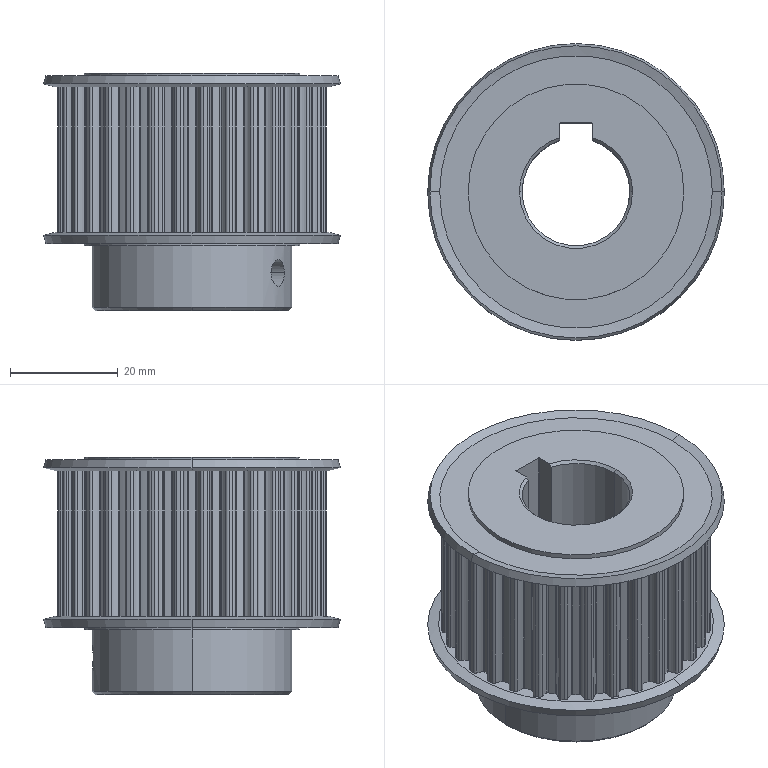Part | SolidWorks | features BaseBody 1 | 1 solid | 328 faces | box 55 x 55 x 44 mm | volume 56659 mm3 | cylinder 300 | cone 18 | plane 10 | commonest cylinder face diameters 1.1 x78 0.5 x74 6.55 x68 46.43 x33 49.97 x32 4.917 x4